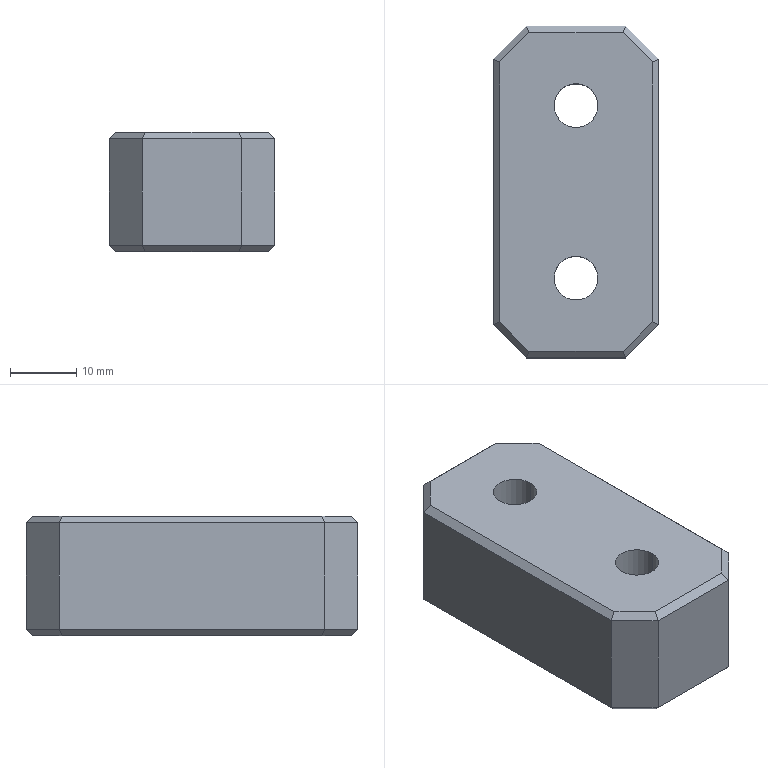Part | Creo | 1 solid | 36 faces | box 25 x 50 x 18 mm | volume 19381 mm3 | plane 28 | cylinder 8 | commonest cylinder face diameters 6.6 x4 11 x4
STEP:
#1=CARTESIAN_POINT('',(55.086,-82.005,-348.));
#2=VERTEX_POINT('',#1);
#3=CARTESIAN_POINT('',(40.914,-82.005,-348.));
#4=VERTEX_POINT('',#3);
#5=CARTESIAN_POINT('',(55.086,-82.005,-348.));
#6=DIRECTION('',(-1.,0.,0.));
#7=VECTOR('',#6,14.172);
#8=LINE('',#5,#7);
#9=EDGE_CURVE('',#2,#4,#8,.T.);
#10=ORIENTED_EDGE('',*,*,#9,.T.);
#11=CARTESIAN_POINT('',(36.5,-77.59,-348.));
#12=VERTEX_POINT('',#11);
#13=CARTESIAN_POINT('',(36.5,-77.59,-348.));
#14=DIRECTION('',(0.7071,-0.7071,0.));
#15=VECTOR('',#14,6.243);
#16=LINE('',#13,#15);
#17=EDGE_CURVE('',#12,#4,#16,.T.);
#18=ORIENTED_EDGE('',*,*,#17,.F.);
#19=CARTESIAN_POINT('',(36.5,-38.419,-348.));
#20=VERTEX_POINT('',#19);
#21=CARTESIAN_POINT('',(36.5,-77.59,-348.));
#22=DIRECTION('',(0.,1.,0.));
#23=VECTOR('',#22,39.172);
#24=LINE('',#21,#23);
#25=EDGE_CURVE('',#12,#20,#24,.T.);
#26=ORIENTED_EDGE('',*,*,#25,.T.);
#27=CARTESIAN_POINT('',(40.914,-34.005,-348.));
#28=VERTEX_POINT('',#27);
#29=CARTESIAN_POINT('',(40.914,-34.005,-348.));
#30=DIRECTION('',(-0.7071,-0.7071,0.));
#31=VECTOR('',#30,6.243);
#32=LINE('',#29,#31);
#33=EDGE_CURVE('',#28,#20,#32,.T.);
#34=ORIENTED_EDGE('',*,*,#33,.F.);
#35=CARTESIAN_POINT('',(55.086,-34.005,-348.));
#36=VERTEX_POINT('',#35);
#37=CARTESIAN_POINT('',(40.914,-34.005,-348.));
#38=DIRECTION('',(1.,0.,0.));
#39=VECTOR('',#38,14.172);
#40=LINE('',#37,#39);
#41=EDGE_CURVE('',#28,#36,#40,.T.);
#42=ORIENTED_EDGE('',*,*,#41,.T.);
#43=CARTESIAN_POINT('',(59.5,-38.419,-348.));
#44=VERTEX_POINT('',#43);
#45=CARTESIAN_POINT('',(59.5,-38.419,-348.));
#46=DIRECTION('',(-0.7071,0.7071,0.));
#47=VECTOR('',#46,6.243);
#48=LINE('',#45,#47);
#49=EDGE_CURVE('',#44,#36,#48,.T.);
#50=ORIENTED_EDGE('',*,*,#49,.F.);
#51=CARTESIAN_POINT('',(59.5,-77.59,-348.));
#52=VERTEX_POINT('',#51);
#53=CARTESIAN_POINT('',(59.5,-38.419,-348.));
#54=DIRECTION('',(0.,-1.,0.));
#55=VECTOR('',#54,39.172);
#56=LINE('',#53,#55);
#57=EDGE_CURVE('',#44,#52,#56,.T.);
#58=ORIENTED_EDGE('',*,*,#57,.T.);
#59=CARTESIAN_POINT('',(55.086,-82.005,-348.));
#60=DIRECTION('',(0.7071,0.7071,0.));
#61=VECTOR('',#60,6.243);
#62=LINE('',#59,#61);
#63=EDGE_CURVE('',#2,#52,#62,.T.);
#64=ORIENTED_EDGE('',*,*,#63,.F.);
#65=EDGE_LOOP('',(#10,#18,#26,#34,#42,#50,#58,#64));
#66=FACE_OUTER_BOUND('',#65,.F.);
#67=CARTESIAN_POINT('',(44.7,-71.005,-348.));
#68=VERTEX_POINT('',#67);
#69=CARTESIAN_POINT('',(51.3,-71.005,-348.));
#70=VERTEX_POINT('',#69);
#71=CARTESIAN_POINT('',(48.,-71.005,-348.));
#72=DIRECTION('',(0.,0.,-1.));
#73=DIRECTION('',(-1.,0.,0.));
#74=AXIS2_PLACEMENT_3D('',#71,#72,#73);
#75=CIRCLE('',#74,3.3);
#76=EDGE_CURVE('',#68,#70,#75,.T.);
#77=ORIENTED_EDGE('',*,*,#76,.F.);
#78=CARTESIAN_POINT('',(48.,-71.005,-348.));
#79=DIRECTION('',(0.,0.,-1.));
#80=DIRECTION('',(1.,0.,0.));
#81=AXIS2_PLACEMENT_3D('',#78,#79,#80);
#82=CIRCLE('',#81,3.3);
#83=EDGE_CURVE('',#70,#68,#82,.T.);
#84=ORIENTED_EDGE('',*,*,#83,.F.);
#85=EDGE_LOOP('',(#77,#84));
#86=FACE_BOUND('',#85,.F.);
#87=CARTESIAN_POINT('',(44.7,-45.005,-348.));
#88=VERTEX_POINT('',#87);
#89=CARTESIAN_POINT('',(51.3,-45.005,-348.));
#90=VERTEX_POINT('',#89);
#91=CARTESIAN_POINT('',(48.,-45.005,-348.));
#92=DIRECTION('',(0.,0.,-1.));
#93=DIRECTION('',(-1.,0.,0.));
#94=AXIS2_PLACEMENT_3D('',#91,#92,#93);
#95=CIRCLE('',#94,3.3);
#96=EDGE_CURVE('',#88,#90,#95,.T.);
#97=ORIENTED_EDGE('',*,*,#96,.F.);
#98=CARTESIAN_POINT('',(48.,-45.005,-348.));
#99=DIRECTION('',(0.,0.,-1.));
#100=DIRECTION('',(1.,0.,0.));
#101=AXIS2_PLACEMENT_3D('',#98,#99,#100);
#102=CIRCLE('',#101,3.3);
#103=EDGE_CURVE('',#90,#88,#102,.T.);
#104=ORIENTED_EDGE('',*,*,#103,.F.);
#105=EDGE_LOOP('',(#97,#104));
#106=FACE_BOUND('',#105,.F.);
#107=CARTESIAN_POINT('',(48.,-58.005,-348.));
#108=DIRECTION('',(0.,0.,1.));
#109=DIRECTION('',(0.,1.,0.));
#110=AXIS2_PLACEMENT_3D('',#107,#108,#109);
#111=PLANE('',#110);
#112=ADVANCED_FACE('',(#66,#86,#106),#111,.T.);
#113=ORIENTED_EDGE('',*,*,#76,.T.);
#114=CARTESIAN_POINT('',(51.3,-71.005,-359.));
#115=VERTEX_POINT('',#114);
#116=CARTESIAN_POINT('',(51.3,-71.005,-348.));
#117=DIRECTION('',(0.,0.,-1.));
#118=VECTOR('',#117,11.);
#119=LINE('',#116,#118);
#120=EDGE_CURVE('',#70,#115,#119,.T.);
#121=ORIENTED_EDGE('',*,*,#120,.T.);
#122=CARTESIAN_POINT('',(44.7,-71.005,-359.));
#123=VERTEX_POINT('',#122);
#124=CARTESIAN_POINT('',(48.,-71.005,-359.));
#125=DIRECTION('',(0.,0.,1.));
#126=DIRECTION('',(1.,0.,0.));
#127=AXIS2_PLACEMENT_3D('',#124,#125,#126);
#128=CIRCLE('',#127,3.3);
#129=EDGE_CURVE('',#115,#123,#128,.T.);
#130=ORIENTED_EDGE('',*,*,#129,.T.);
#131=CARTESIAN_POINT('',(44.7,-71.005,-348.));
#132=DIRECTION('',(0.,0.,-1.));
#133=VECTOR('',#132,11.);
#134=LINE('',#131,#133);
#135=EDGE_CURVE('',#68,#123,#134,.T.);
#136=ORIENTED_EDGE('',*,*,#135,.F.);
#137=EDGE_LOOP('',(#113,#121,#130,#136));
#138=FACE_OUTER_BOUND('',#137,.F.);
#139=CARTESIAN_POINT('',(48.,-71.005,-366.));
#140=DIRECTION('',(0.,0.,-1.));
#141=DIRECTION('',(-1.,0.,0.));
#142=AXIS2_PLACEMENT_3D('',#139,#140,#141);
#143=CYLINDRICAL_SURFACE('',#142,3.3);
#144=ADVANCED_FACE('',(#138),#143,.F.);
#145=ORIENTED_EDGE('',*,*,#83,.T.);
#146=ORIENTED_EDGE('',*,*,#135,.T.);
#147=CARTESIAN_POINT('',(48.,-71.005,-359.));
#148=DIRECTION('',(0.,0.,1.));
#149=DIRECTION('',(-1.,0.,0.));
#150=AXIS2_PLACEMENT_3D('',#147,#148,#149);
#151=CIRCLE('',#150,3.3);
#152=EDGE_CURVE('',#123,#115,#151,.T.);
#153=ORIENTED_EDGE('',*,*,#152,.T.);
#154=ORIENTED_EDGE('',*,*,#120,.F.);
#155=EDGE_LOOP('',(#145,#146,#153,#154));
#156=FACE_OUTER_BOUND('',#155,.F.);
#157=CARTESIAN_POINT('',(48.,-71.005,-366.));
#158=DIRECTION('',(0.,0.,-1.));
#159=DIRECTION('',(-1.,0.,0.));
#160=AXIS2_PLACEMENT_3D('',#157,#158,#159);
#161=CYLINDRICAL_SURFACE('',#160,3.3);
#162=ADVANCED_FACE('',(#156),#161,.F.);
#163=CARTESIAN_POINT('',(48.,-65.505,-359.));
#164=VERTEX_POINT('',#163);
#165=CARTESIAN_POINT('',(48.,-76.505,-359.));
#166=VERTEX_POINT('',#165);
#167=CARTESIAN_POINT('',(48.,-71.005,-359.));
#168=DIRECTION('',(0.,0.,-1.));
#169=DIRECTION('',(0.,1.,0.));
#170=AXIS2_PLACEMENT_3D('',#167,#168,#169);
#171=CIRCLE('',#170,5.5);
#172=EDGE_CURVE('',#164,#166,#171,.T.);
#173=ORIENTED_EDGE('',*,*,#172,.F.);
#174=CARTESIAN_POINT('',(48.,-71.005,-359.));
#175=DIRECTION('',(0.,0.,-1.));
#176=DIRECTION('',(0.,-1.,0.));
#177=AXIS2_PLACEMENT_3D('',#174,#175,#176);
#178=CIRCLE('',#177,5.5);
#179=EDGE_CURVE('',#166,#164,#178,.T.);
#180=ORIENTED_EDGE('',*,*,#179,.F.);
#181=EDGE_LOOP('',(#173,#180));
#182=FACE_OUTER_BOUND('',#181,.F.);
#183=ORIENTED_EDGE('',*,*,#152,.F.);
#184=ORIENTED_EDGE('',*,*,#129,.F.);
#185=EDGE_LOOP('',(#183,#184));
#186=FACE_BOUND('',#185,.F.);
#187=CARTESIAN_POINT('',(48.,-71.005,-359.));
#188=DIRECTION('',(0.,0.,1.));
#189=DIRECTION('',(0.,1.,0.));
#190=AXIS2_PLACEMENT_3D('',#187,#188,#189);
#191=PLANE('',#190);
#192=ADVANCED_FACE('',(#182,#186),#191,.F.);
#193=ORIENTED_EDGE('',*,*,#172,.T.);
#194=CARTESIAN_POINT('',(48.,-76.505,-366.));
#195=VERTEX_POINT('',#194);
#196=CARTESIAN_POINT('',(48.,-76.505,-366.));
#197=DIRECTION('',(0.,0.,1.));
#198=VECTOR('',#197,7.);
#199=LINE('',#196,#198);
#200=EDGE_CURVE('',#195,#166,#199,.T.);
#201=ORIENTED_EDGE('',*,*,#200,.F.);
#202=CARTESIAN_POINT('',(53.5,-71.005,-366.));
#203=VERTEX_POINT('',#202);
#204=CARTESIAN_POINT('',(48.,-71.005,-366.));
#205=DIRECTION('',(0.,0.,1.));
#206=DIRECTION('',(0.,-1.,0.));
#207=AXIS2_PLACEMENT_3D('',#204,#205,#206);
#208=CIRCLE('',#207,5.5);
#209=EDGE_CURVE('',#195,#203,#208,.T.);
#210=ORIENTED_EDGE('',*,*,#209,.T.);
#211=CARTESIAN_POINT('',(48.,-65.505,-366.));
#212=VERTEX_POINT('',#211);
#213=CARTESIAN_POINT('',(48.,-71.005,-366.));
#214=DIRECTION('',(0.,0.,1.));
#215=DIRECTION('',(1.,0.,0.));
#216=AXIS2_PLACEMENT_3D('',#213,#214,#215);
#217=CIRCLE('',#216,5.5);
#218=EDGE_CURVE('',#203,#212,#217,.T.);
#219=ORIENTED_EDGE('',*,*,#218,.T.);
#220=CARTESIAN_POINT('',(48.,-65.505,-366.));
#221=DIRECTION('',(0.,0.,1.));
#222=VECTOR('',#221,7.);
#223=LINE('',#220,#222);
#224=EDGE_CURVE('',#212,#164,#223,.T.);
#225=ORIENTED_EDGE('',*,*,#224,.T.);
#226=EDGE_LOOP('',(#193,#201,#210,#219,#225));
#227=FACE_OUTER_BOUND('',#226,.F.);
#228=CARTESIAN_POINT('',(48.,-71.005,-372.));
#229=DIRECTION('',(0.,0.,1.));
#230=DIRECTION('',(0.,1.,0.));
#231=AXIS2_PLACEMENT_3D('',#228,#229,#230);
#232=CYLINDRICAL_SURFACE('',#231,5.5);
#233=ADVANCED_FACE('',(#227),#232,.F.);
#234=ORIENTED_EDGE('',*,*,#179,.T.);
#235=ORIENTED_EDGE('',*,*,#224,.F.);
#236=CARTESIAN_POINT('',(42.5,-71.005,-366.));
#237=VERTEX_POINT('',#236);
#238=CARTESIAN_POINT('',(48.,-71.005,-366.));
#239=DIRECTION('',(0.,0.,1.));
#240=DIRECTION('',(0.,1.,0.));
#241=AXIS2_PLACEMENT_3D('',#238,#239,#240);
#242=CIRCLE('',#241,5.5);
#243=EDGE_CURVE('',#212,#237,#242,.T.);
#244=ORIENTED_EDGE('',*,*,#243,.T.);
#245=CARTESIAN_POINT('',(48.,-71.005,-366.));
#246=DIRECTION('',(0.,0.,1.));
#247=DIRECTION('',(-1.,0.,0.));
#248=AXIS2_PLACEMENT_3D('',#245,#246,#247);
#249=CIRCLE('',#248,5.5);
#250=EDGE_CURVE('',#237,#195,#249,.T.);
#251=ORIENTED_EDGE('',*,*,#250,.T.);
#252=ORIENTED_EDGE('',*,*,#200,.T.);
#253=EDGE_LOOP('',(#234,#235,#244,#251,#252));
#254=FACE_OUTER_BOUND('',#253,.F.);
#255=CARTESIAN_POINT('',(48.,-71.005,-372.));
#256=DIRECTION('',(0.,0.,1.));
#257=DIRECTION('',(0.,1.,0.));
#258=AXIS2_PLACEMENT_3D('',#255,#256,#257);
#259=CYLINDRICAL_SURFACE('',#258,5.5);
#260=ADVANCED_FACE('',(#254),#259,.F.);
#261=CARTESIAN_POINT('',(59.5,-77.59,-366.));
#262=VERTEX_POINT('',#261);
#263=CARTESIAN_POINT('',(59.5,-38.419,-366.));
#264=VERTEX_POINT('',#263);
#265=CARTESIAN_POINT('',(59.5,-77.59,-366.));
#266=DIRECTION('',(0.,1.,0.));
#267=VECTOR('',#266,39.172);
#268=LINE('',#265,#267);
#269=EDGE_CURVE('',#262,#264,#268,.T.);
#270=ORIENTED_EDGE('',*,*,#269,.T.);
#271=CARTESIAN_POINT('',(55.086,-34.005,-366.));
#272=VERTEX_POINT('',#271);
#273=CARTESIAN_POINT('',(55.086,-34.005,-366.));
#274=DIRECTION('',(0.7071,-0.7071,0.));
#275=VECTOR('',#274,6.243);
#276=LINE('',#273,#275);
#277=EDGE_CURVE('',#272,#264,#276,.T.);
#278=ORIENTED_EDGE('',*,*,#277,.F.);
#279=CARTESIAN_POINT('',(40.914,-34.005,-366.));
#280=VERTEX_POINT('',#279);
#281=CARTESIAN_POINT('',(55.086,-34.005,-366.));
#282=DIRECTION('',(-1.,0.,0.));
#283=VECTOR('',#282,14.172);
#284=LINE('',#281,#283);
#285=EDGE_CURVE('',#272,#280,#284,.T.);
#286=ORIENTED_EDGE('',*,*,#285,.T.);
#287=CARTESIAN_POINT('',(36.5,-38.419,-366.));
#288=VERTEX_POINT('',#287);
#289=CARTESIAN_POINT('',(36.5,-38.419,-366.));
#290=DIRECTION('',(0.7071,0.7071,0.));
#291=VECTOR('',#290,6.243);
#292=LINE('',#289,#291);
#293=EDGE_CURVE('',#288,#280,#292,.T.);
#294=ORIENTED_EDGE('',*,*,#293,.F.);
#295=CARTESIAN_POINT('',(36.5,-77.59,-366.));
#296=VERTEX_POINT('',#295);
#297=CARTESIAN_POINT('',(36.5,-38.419,-366.));
#298=DIRECTION('',(0.,-1.,0.));
#299=VECTOR('',#298,39.172);
#300=LINE('',#297,#299);
#301=EDGE_CURVE('',#288,#296,#300,.T.);
#302=ORIENTED_EDGE('',*,*,#301,.T.);
#303=CARTESIAN_POINT('',(40.914,-82.005,-366.));
#304=VERTEX_POINT('',#303);
#305=CARTESIAN_POINT('',(40.914,-82.005,-366.));
#306=DIRECTION('',(-0.7071,0.7071,0.));
#307=VECTOR('',#306,6.243);
#308=LINE('',#305,#307);
#309=EDGE_CURVE('',#304,#296,#308,.T.);
#310=ORIENTED_EDGE('',*,*,#309,.F.);
#311=CARTESIAN_POINT('',(55.086,-82.005,-366.));
#312=VERTEX_POINT('',#311);
#313=CARTESIAN_POINT('',(40.914,-82.005,-366.));
#314=DIRECTION('',(1.,0.,0.));
#315=VECTOR('',#314,14.172);
#316=LINE('',#313,#315);
#317=EDGE_CURVE('',#304,#312,#316,.T.);
#318=ORIENTED_EDGE('',*,*,#317,.T.);
#319=CARTESIAN_POINT('',(59.5,-77.59,-366.));
#320=DIRECTION('',(-0.7071,-0.7071,0.));
#321=VECTOR('',#320,6.243);
#322=LINE('',#319,#321);
#323=EDGE_CURVE('',#262,#312,#322,.T.);
#324=ORIENTED_EDGE('',*,*,#323,.F.);
#325=EDGE_LOOP('',(#270,#278,#286,#294,#302,#310,#318,#324));
#326=FACE_OUTER_BOUND('',#325,.F.);
#327=CARTESIAN_POINT('',(53.5,-45.005,-366.));
#328=VERTEX_POINT('',#327);
#329=CARTESIAN_POINT('',(48.,-39.505,-366.));
#330=VERTEX_POINT('',#329);
#331=CARTESIAN_POINT('',(48.,-45.005,-366.));
#332=DIRECTION('',(0.,0.,1.));
#333=DIRECTION('',(1.,0.,0.));
#334=AXIS2_PLACEMENT_3D('',#331,#332,#333);
#335=CIRCLE('',#334,5.5);
#336=EDGE_CURVE('',#328,#330,#335,.T.);
#337=ORIENTED_EDGE('',*,*,#336,.F.);
#338=CARTESIAN_POINT('',(48.,-50.505,-366.));
#339=VERTEX_POINT('',#338);
#340=CARTESIAN_POINT('',(48.,-45.005,-366.));
#341=DIRECTION('',(0.,0.,1.));
#342=DIRECTION('',(0.,-1.,0.));
#343=AXIS2_PLACEMENT_3D('',#340,#341,#342);
#344=CIRCLE('',#343,5.5);
#345=EDGE_CURVE('',#339,#328,#344,.T.);
#346=ORIENTED_EDGE('',*,*,#345,.F.);
#347=CARTESIAN_POINT('',(42.5,-45.005,-366.));
#348=VERTEX_POINT('',#347);
#349=CARTESIAN_POINT('',(48.,-45.005,-366.));
#350=DIRECTION('',(0.,0.,1.));
#351=DIRECTION('',(-1.,0.,0.));
#352=AXIS2_PLACEMENT_3D('',#349,#350,#351);
#353=CIRCLE('',#352,5.5);
#354=EDGE_CURVE('',#348,#339,#353,.T.);
#355=ORIENTED_EDGE('',*,*,#354,.F.);
#356=CARTESIAN_POINT('',(48.,-45.005,-366.));
#357=DIRECTION('',(0.,0.,1.));
#358=DIRECTION('',(0.,1.,0.));
#359=AXIS2_PLACEMENT_3D('',#356,#357,#358);
#360=CIRCLE('',#359,5.5);
#361=EDGE_CURVE('',#330,#348,#360,.T.);
#362=ORIENTED_EDGE('',*,*,#361,.F.);
#363=EDGE_LOOP('',(#337,#346,#355,#362));
#364=FACE_BOUND('',#363,.F.);
#365=ORIENTED_EDGE('',*,*,#218,.F.);
#366=ORIENTED_EDGE('',*,*,#209,.F.);
#367=ORIENTED_EDGE('',*,*,#250,.F.);
#368=ORIENTED_EDGE('',*,*,#243,.F.);
#369=EDGE_LOOP('',(#365,#366,#367,#368));
#370=FACE_BOUND('',#369,.F.);
#371=CARTESIAN_POINT('',(10.,-0.004699,-366.));
#372=DIRECTION('',(0.,0.,1.));
#373=DIRECTION('',(0.,1.,0.));
#374=AXIS2_PLACEMENT_3D('',#371,#372,#373);
#375=PLANE('',#374);
#376=ADVANCED_FACE('',(#326,#364,#370),#375,.F.);
#377=CARTESIAN_POINT('',(60.5,-38.005,-365.));
#378=VERTEX_POINT('',#377);
#379=CARTESIAN_POINT('',(60.5,-38.005,-365.));
#380=DIRECTION('',(-0.6786,-0.2811,-0.6786));
#381=VECTOR('',#380,1.474);
#382=LINE('',#379,#381);
#383=EDGE_CURVE('',#378,#264,#382,.T.);
#384=ORIENTED_EDGE('',*,*,#383,.T.);
#385=ORIENTED_EDGE('',*,*,#269,.F.);
#386=CARTESIAN_POINT('',(60.5,-78.005,-365.));
#387=VERTEX_POINT('',#386);
#388=CARTESIAN_POINT('',(60.5,-78.005,-365.));
#389=DIRECTION('',(-0.6786,0.2811,-0.6786));
#390=VECTOR('',#389,1.474);
#391=LINE('',#388,#390);
#392=EDGE_CURVE('',#387,#262,#391,.T.);
#393=ORIENTED_EDGE('',*,*,#392,.F.);
#394=CARTESIAN_POINT('',(60.5,-38.005,-365.));
#395=DIRECTION('',(0.,-1.,0.));
#396=VECTOR('',#395,40.);
#397=LINE('',#394,#396);
#398=EDGE_CURVE('',#378,#387,#397,.T.);
#399=ORIENTED_EDGE('',*,*,#398,.F.);
#400=EDGE_LOOP('',(#384,#385,#393,#399));
#401=FACE_OUTER_BOUND('',#400,.F.);
#402=CARTESIAN_POINT('',(60.5,-88.005,-365.));
#403=DIRECTION('',(0.7071,0.,-0.7071));
#404=DIRECTION('',(0.,1.,0.));
#405=AXIS2_PLACEMENT_3D('',#402,#403,#404);
#406=PLANE('',#405);
#407=ADVANCED_FACE('',(#401),#406,.T.);
#408=CARTESIAN_POINT('',(55.5,-33.005,-365.));
#409=VERTEX_POINT('',#408);
#410=CARTESIAN_POINT('',(55.5,-33.005,-365.));
#411=DIRECTION('',(-0.2811,-0.6786,-0.6786));
#412=VECTOR('',#411,1.474);
#413=LINE('',#410,#412);
#414=EDGE_CURVE('',#409,#272,#413,.T.);
#415=ORIENTED_EDGE('',*,*,#414,.T.);
#416=ORIENTED_EDGE('',*,*,#277,.T.);
#417=ORIENTED_EDGE('',*,*,#383,.F.);
#418=CARTESIAN_POINT('',(55.5,-33.005,-365.));
#419=DIRECTION('',(0.7071,-0.7071,0.));
#420=VECTOR('',#419,7.071);
#421=LINE('',#418,#420);
#422=EDGE_CURVE('',#409,#378,#421,.T.);
#423=ORIENTED_EDGE('',*,*,#422,.F.);
#424=EDGE_LOOP('',(#415,#416,#417,#423));
#425=FACE_OUTER_BOUND('',#424,.F.);
#426=CARTESIAN_POINT('',(15.543,5.538,-366.));
#427=DIRECTION('',(-0.5,-0.5,0.7071));
#428=DIRECTION('',(-0.7071,0.7071,0.));
#429=AXIS2_PLACEMENT_3D('',#426,#427,#428);
#430=PLANE('',#429);
#431=ADVANCED_FACE('',(#425),#430,.F.);
#432=CARTESIAN_POINT('',(40.5,-33.005,-365.));
#433=VERTEX_POINT('',#432);
#434=CARTESIAN_POINT('',(40.5,-33.005,-365.));
#435=DIRECTION('',(0.2811,-0.6786,-0.6786));
#436=VECTOR('',#435,1.474);
#437=LINE('',#434,#436);
#438=EDGE_CURVE('',#433,#280,#437,.T.);
#439=ORIENTED_EDGE('',*,*,#438,.T.);
#440=ORIENTED_EDGE('',*,*,#285,.F.);
#441=ORIENTED_EDGE('',*,*,#414,.F.);
#442=CARTESIAN_POINT('',(40.5,-33.005,-365.));
#443=DIRECTION('',(1.,0.,0.));
#444=VECTOR('',#443,15.);
#445=LINE('',#442,#444);
#446=EDGE_CURVE('',#433,#409,#445,.T.);
#447=ORIENTED_EDGE('',*,*,#446,.F.);
#448=EDGE_LOOP('',(#439,#440,#441,#447));
#449=FACE_OUTER_BOUND('',#448,.F.);
#450=CARTESIAN_POINT('',(63.,-33.005,-365.));
#451=DIRECTION('',(0.,0.7071,-0.7071));
#452=DIRECTION('',(-1.,0.,0.));
#453=AXIS2_PLACEMENT_3D('',#450,#451,#452);
#454=PLANE('',#453);
#455=ADVANCED_FACE('',(#449),#454,.T.);
#456=CARTESIAN_POINT('',(35.5,-38.005,-365.));
#457=VERTEX_POINT('',#456);
#458=CARTESIAN_POINT('',(36.5,-38.419,-366.));
#459=DIRECTION('',(-0.6786,0.2811,0.6786));
#460=VECTOR('',#459,1.474);
#461=LINE('',#458,#460);
#462=EDGE_CURVE('',#288,#457,#461,.T.);
#463=ORIENTED_EDGE('',*,*,#462,.F.);
#464=ORIENTED_EDGE('',*,*,#293,.T.);
#465=ORIENTED_EDGE('',*,*,#438,.F.);
#466=CARTESIAN_POINT('',(35.5,-38.005,-365.));
#467=DIRECTION('',(0.7071,0.7071,0.));
#468=VECTOR('',#467,7.071);
#469=LINE('',#466,#468);
#470=EDGE_CURVE('',#457,#433,#469,.T.);
#471=ORIENTED_EDGE('',*,*,#470,.F.);
#472=EDGE_LOOP('',(#463,#464,#465,#471));
#473=FACE_OUTER_BOUND('',#472,.F.);
#474=CARTESIAN_POINT('',(42.457,-32.462,-366.));
#475=DIRECTION('',(0.5,-0.5,0.7071));
#476=DIRECTION('',(-0.7071,-0.7071,0.));
#477=AXIS2_PLACEMENT_3D('',#474,#475,#476);
#478=PLANE('',#477);
#479=ADVANCED_FACE('',(#473),#478,.F.);
#480=ORIENTED_EDGE('',*,*,#462,.T.);
#481=CARTESIAN_POINT('',(35.5,-78.005,-365.));
#482=VERTEX_POINT('',#481);
#483=CARTESIAN_POINT('',(35.5,-78.005,-365.));
#484=DIRECTION('',(0.,1.,0.));
#485=VECTOR('',#484,40.);
#486=LINE('',#483,#485);
#487=EDGE_CURVE('',#482,#457,#486,.T.);
#488=ORIENTED_EDGE('',*,*,#487,.F.);
#489=CARTESIAN_POINT('',(36.5,-77.59,-366.));
#490=DIRECTION('',(-0.6786,-0.2811,0.6786));
#491=VECTOR('',#490,1.474);
#492=LINE('',#489,#491);
#493=EDGE_CURVE('',#296,#482,#492,.T.);
#494=ORIENTED_EDGE('',*,*,#493,.F.);
#495=ORIENTED_EDGE('',*,*,#301,.F.);
#496=EDGE_LOOP('',(#480,#488,#494,#495));
#497=FACE_OUTER_BOUND('',#496,.F.);
#498=CARTESIAN_POINT('',(35.5,-28.005,-365.));
#499=DIRECTION('',(-0.7071,0.,-0.7071));
#500=DIRECTION('',(0.,-1.,0.));
#501=AXIS2_PLACEMENT_3D('',#498,#499,#500);
#502=PLANE('',#501);
#503=ADVANCED_FACE('',(#497),#502,.T.);
#504=CARTESIAN_POINT('',(35.5,-38.005,-349.));
#505=VERTEX_POINT('',#504);
#506=CARTESIAN_POINT('',(35.5,-38.005,-365.));
#507=DIRECTION('',(0.,0.,1.));
#508=VECTOR('',#507,16.);
#509=LINE('',#506,#508);
#510=EDGE_CURVE('',#457,#505,#509,.T.);
#511=ORIENTED_EDGE('',*,*,#510,.T.);
#512=CARTESIAN_POINT('',(35.5,-78.005,-349.));
#513=VERTEX_POINT('',#512);
#514=CARTESIAN_POINT('',(35.5,-38.005,-349.));
#515=DIRECTION('',(0.,-1.,0.));
#516=VECTOR('',#515,40.);
#517=LINE('',#514,#516);
#518=EDGE_CURVE('',#505,#513,#517,.T.);
#519=ORIENTED_EDGE('',*,*,#518,.T.);
#520=CARTESIAN_POINT('',(35.5,-78.005,-349.));
#521=DIRECTION('',(0.,0.,-1.));
#522=VECTOR('',#521,16.);
#523=LINE('',#520,#522);
#524=EDGE_CURVE('',#513,#482,#523,.T.);
#525=ORIENTED_EDGE('',*,*,#524,.T.);
#526=ORIENTED_EDGE('',*,*,#487,.T.);
#527=EDGE_LOOP('',(#511,#519,#525,#526));
#528=FACE_OUTER_BOUND('',#527,.F.);
#529=CARTESIAN_POINT('',(35.5,-28.005,-354.));
#530=DIRECTION('',(-1.,0.,0.));
#531=DIRECTION('',(0.,-1.,0.));
#532=AXIS2_PLACEMENT_3D('',#529,#530,#531);
#533=PLANE('',#532);
#534=ADVANCED_FACE('',(#528),#533,.T.);
#535=CARTESIAN_POINT('',(40.5,-33.005,-349.));
#536=VERTEX_POINT('',#535);
#537=CARTESIAN_POINT('',(40.5,-33.005,-349.));
#538=DIRECTION('',(0.,0.,-1.));
#539=VECTOR('',#538,16.);
#540=LINE('',#537,#539);
#541=EDGE_CURVE('',#536,#433,#540,.T.);
#542=ORIENTED_EDGE('',*,*,#541,.F.);
#543=CARTESIAN_POINT('',(40.5,-33.005,-349.));
#544=DIRECTION('',(-0.7071,-0.7071,0.));
#545=VECTOR('',#544,7.071);
#546=LINE('',#543,#545);
#547=EDGE_CURVE('',#536,#505,#546,.T.);
#548=ORIENTED_EDGE('',*,*,#547,.T.);
#549=ORIENTED_EDGE('',*,*,#510,.F.);
#550=ORIENTED_EDGE('',*,*,#470,.T.);
#551=EDGE_LOOP('',(#542,#548,#549,#550));
#552=FACE_OUTER_BOUND('',#551,.F.);
#553=CARTESIAN_POINT('',(40.5,-33.005,-354.));
#554=DIRECTION('',(0.7071,-0.7071,0.));
#555=DIRECTION('',(0.,0.,-1.));
#556=AXIS2_PLACEMENT_3D('',#553,#554,#555);
#557=PLANE('',#556);
#558=ADVANCED_FACE('',(#552),#557,.F.);
#559=CARTESIAN_POINT('',(55.5,-33.005,-349.));
#560=VERTEX_POINT('',#559);
#561=CARTESIAN_POINT('',(55.5,-33.005,-365.));
#562=DIRECTION('',(0.,0.,1.));
#563=VECTOR('',#562,16.);
#564=LINE('',#561,#563);
#565=EDGE_CURVE('',#409,#560,#564,.T.);
#566=ORIENTED_EDGE('',*,*,#565,.T.);
#567=CARTESIAN_POINT('',(55.5,-33.005,-349.));
#568=DIRECTION('',(-1.,0.,0.));
#569=VECTOR('',#568,15.);
#570=LINE('',#567,#569);
#571=EDGE_CURVE('',#560,#536,#570,.T.);
#572=ORIENTED_EDGE('',*,*,#571,.T.);
#573=ORIENTED_EDGE('',*,*,#541,.T.);
#574=ORIENTED_EDGE('',*,*,#446,.T.);
#575=EDGE_LOOP('',(#566,#572,#573,#574));
#576=FACE_OUTER_BOUND('',#575,.F.);
#577=CARTESIAN_POINT('',(63.,-33.005,-354.));
#578=DIRECTION('',(0.,1.,0.));
#579=DIRECTION('',(-1.,0.,0.));
#580=AXIS2_PLACEMENT_3D('',#577,#578,#579);
#581=PLANE('',#580);
#582=ADVANCED_FACE('',(#576),#581,.T.);
#583=CARTESIAN_POINT('',(60.5,-38.005,-349.));
#584=VERTEX_POINT('',#583);
#585=CARTESIAN_POINT('',(60.5,-38.005,-349.));
#586=DIRECTION('',(0.,0.,-1.));
#587=VECTOR('',#586,16.);
#588=LINE('',#585,#587);
#589=EDGE_CURVE('',#584,#378,#588,.T.);
#590=ORIENTED_EDGE('',*,*,#589,.F.);
#591=CARTESIAN_POINT('',(60.5,-38.005,-349.));
#592=DIRECTION('',(-0.7071,0.7071,0.));
#593=VECTOR('',#592,7.071);
#594=LINE('',#591,#593);
#595=EDGE_CURVE('',#584,#560,#594,.T.);
#596=ORIENTED_EDGE('',*,*,#595,.T.);
#597=ORIENTED_EDGE('',*,*,#565,.F.);
#598=ORIENTED_EDGE('',*,*,#422,.T.);
#599=EDGE_LOOP('',(#590,#596,#597,#598));
#600=FACE_OUTER_BOUND('',#599,.F.);
#601=CARTESIAN_POINT('',(60.5,-38.005,-354.));
#602=DIRECTION('',(-0.7071,-0.7071,0.));
#603=DIRECTION('',(0.,0.,-1.));
#604=AXIS2_PLACEMENT_3D('',#601,#602,#603);
#605=PLANE('',#604);
#606=ADVANCED_FACE('',(#600),#605,.F.);
#607=CARTESIAN_POINT('',(60.5,-78.005,-349.));
#608=VERTEX_POINT('',#607);
#609=CARTESIAN_POINT('',(60.5,-78.005,-365.));
#610=DIRECTION('',(0.,0.,1.));
#611=VECTOR('',#610,16.);
#612=LINE('',#609,#611);
#613=EDGE_CURVE('',#387,#608,#612,.T.);
#614=ORIENTED_EDGE('',*,*,#613,.T.);
#615=CARTESIAN_POINT('',(60.5,-78.005,-349.));
#616=DIRECTION('',(0.,1.,0.));
#617=VECTOR('',#616,40.);
#618=LINE('',#615,#617);
#619=EDGE_CURVE('',#608,#584,#618,.T.);
#620=ORIENTED_EDGE('',*,*,#619,.T.);
#621=ORIENTED_EDGE('',*,*,#589,.T.);
#622=ORIENTED_EDGE('',*,*,#398,.T.);
#623=EDGE_LOOP('',(#614,#620,#621,#622));
#624=FACE_OUTER_BOUND('',#623,.F.);
#625=CARTESIAN_POINT('',(60.5,-88.005,-354.));
#626=DIRECTION('',(1.,0.,0.));
#627=DIRECTION('',(0.,1.,0.));
#628=AXIS2_PLACEMENT_3D('',#625,#626,#627);
#629=PLANE('',#628);
#630=ADVANCED_FACE('',(#624),#629,.T.);
#631=CARTESIAN_POINT('',(55.5,-83.005,-349.));
#632=VERTEX_POINT('',#631);
#633=CARTESIAN_POINT('',(55.5,-83.005,-365.));
#634=VERTEX_POINT('',#633);
#635=CARTESIAN_POINT('',(55.5,-83.005,-349.));
#636=DIRECTION('',(0.,0.,-1.));
#637=VECTOR('',#636,16.);
#638=LINE('',#635,#637);
#639=EDGE_CURVE('',#632,#634,#638,.T.);
#640=ORIENTED_EDGE('',*,*,#639,.F.);
#641=CARTESIAN_POINT('',(55.5,-83.005,-349.));
#642=DIRECTION('',(0.7071,0.7071,0.));
#643=VECTOR('',#642,7.071);
#644=LINE('',#641,#643);
#645=EDGE_CURVE('',#632,#608,#644,.T.);
#646=ORIENTED_EDGE('',*,*,#645,.T.);
#647=ORIENTED_EDGE('',*,*,#613,.F.);
#648=CARTESIAN_POINT('',(60.5,-78.005,-365.));
#649=DIRECTION('',(-0.7071,-0.7071,0.));
#650=VECTOR('',#649,7.071);
#651=LINE('',#648,#650);
#652=EDGE_CURVE('',#387,#634,#651,.T.);
#653=ORIENTED_EDGE('',*,*,#652,.T.);
#654=EDGE_LOOP('',(#640,#646,#647,#653));
#655=FACE_OUTER_BOUND('',#654,.F.);
#656=CARTESIAN_POINT('',(55.5,-83.005,-354.));
#657=DIRECTION('',(-0.7071,0.7071,0.));
#658=DIRECTION('',(0.,0.,-1.));
#659=AXIS2_PLACEMENT_3D('',#656,#657,#658);
#660=PLANE('',#659);
#661=ADVANCED_FACE('',(#655),#660,.F.);
#662=CARTESIAN_POINT('',(40.5,-83.005,-365.));
#663=VERTEX_POINT('',#662);
#664=CARTESIAN_POINT('',(40.5,-83.005,-349.));
#665=VERTEX_POINT('',#664);
#666=CARTESIAN_POINT('',(40.5,-83.005,-365.));
#667=DIRECTION('',(0.,0.,1.));
#668=VECTOR('',#667,16.);
#669=LINE('',#666,#668);
#670=EDGE_CURVE('',#663,#665,#669,.T.);
#671=ORIENTED_EDGE('',*,*,#670,.T.);
#672=CARTESIAN_POINT('',(40.5,-83.005,-349.));
#673=DIRECTION('',(1.,0.,0.));
#674=VECTOR('',#673,15.);
#675=LINE('',#672,#674);
#676=EDGE_CURVE('',#665,#632,#675,.T.);
#677=ORIENTED_EDGE('',*,*,#676,.T.);
#678=ORIENTED_EDGE('',*,*,#639,.T.);
#679=CARTESIAN_POINT('',(55.5,-83.005,-365.));
#680=DIRECTION('',(-1.,0.,0.));
#681=VECTOR('',#680,15.);
#682=LINE('',#679,#681);
#683=EDGE_CURVE('',#634,#663,#682,.T.);
#684=ORIENTED_EDGE('',*,*,#683,.T.);
#685=EDGE_LOOP('',(#671,#677,#678,#684));
#686=FACE_OUTER_BOUND('',#685,.F.);
#687=CARTESIAN_POINT('',(33.,-83.005,-354.));
#688=DIRECTION('',(0.,-1.,0.));
#689=DIRECTION('',(1.,0.,0.));
#690=AXIS2_PLACEMENT_3D('',#687,#688,#689);
#691=PLANE('',#690);
#692=ADVANCED_FACE('',(#686),#691,.T.);
#693=ORIENTED_EDGE('',*,*,#524,.F.);
#694=CARTESIAN_POINT('',(35.5,-78.005,-349.));
#695=DIRECTION('',(0.7071,-0.7071,0.));
#696=VECTOR('',#695,7.071);
#697=LINE('',#694,#696);
#698=EDGE_CURVE('',#513,#665,#697,.T.);
#699=ORIENTED_EDGE('',*,*,#698,.T.);
#700=ORIENTED_EDGE('',*,*,#670,.F.);
#701=CARTESIAN_POINT('',(40.5,-83.005,-365.));
#702=DIRECTION('',(-0.7071,0.7071,0.));
#703=VECTOR('',#702,7.071);
#704=LINE('',#701,#703);
#705=EDGE_CURVE('',#663,#482,#704,.T.);
#706=ORIENTED_EDGE('',*,*,#705,.T.);
#707=EDGE_LOOP('',(#693,#699,#700,#706));
#708=FACE_OUTER_BOUND('',#707,.F.);
#709=CARTESIAN_POINT('',(35.5,-78.005,-354.));
#710=DIRECTION('',(0.7071,0.7071,0.));
#711=DIRECTION('',(0.,0.,-1.));
#712=AXIS2_PLACEMENT_3D('',#709,#710,#711);
#713=PLANE('',#712);
#714=ADVANCED_FACE('',(#708),#713,.F.);
#715=CARTESIAN_POINT('',(35.5,-78.005,-349.));
#716=DIRECTION('',(0.6786,0.2811,0.6786));
#717=VECTOR('',#716,1.474);
#718=LINE('',#715,#717);
#719=EDGE_CURVE('',#513,#12,#718,.T.);
#720=ORIENTED_EDGE('',*,*,#719,.T.);
#721=ORIENTED_EDGE('',*,*,#17,.T.);
#722=CARTESIAN_POINT('',(40.5,-83.005,-349.));
#723=DIRECTION('',(0.2811,0.6786,0.6786));
#724=VECTOR('',#723,1.474);
#725=LINE('',#722,#724);
#726=EDGE_CURVE('',#665,#4,#725,.T.);
#727=ORIENTED_EDGE('',*,*,#726,.F.);
#728=ORIENTED_EDGE('',*,*,#698,.F.);
#729=EDGE_LOOP('',(#720,#721,#727,#728));
#730=FACE_OUTER_BOUND('',#729,.F.);
#731=CARTESIAN_POINT('',(32.457,-73.548,-348.));
#732=DIRECTION('',(-0.5,-0.5,0.7071));
#733=DIRECTION('',(0.7071,-0.7071,0.));
#734=AXIS2_PLACEMENT_3D('',#731,#732,#733);
#735=PLANE('',#734);
#736=ADVANCED_FACE('',(#730),#735,.T.);
#737=CARTESIAN_POINT('',(35.5,-38.005,-349.));
#738=DIRECTION('',(0.6786,-0.2811,0.6786));
#739=VECTOR('',#738,1.474);
#740=LINE('',#737,#739);
#741=EDGE_CURVE('',#505,#20,#740,.T.);
#742=ORIENTED_EDGE('',*,*,#741,.T.);
#743=ORIENTED_EDGE('',*,*,#25,.F.);
#744=ORIENTED_EDGE('',*,*,#719,.F.);
#745=ORIENTED_EDGE('',*,*,#518,.F.);
#746=EDGE_LOOP('',(#742,#743,#744,#745));
#747=FACE_OUTER_BOUND('',#746,.F.);
#748=CARTESIAN_POINT('',(35.5,-28.005,-349.));
#749=DIRECTION('',(0.7071,0.,-0.7071));
#750=DIRECTION('',(0.,-1.,0.));
#751=AXIS2_PLACEMENT_3D('',#748,#749,#750);
#752=PLANE('',#751);
#753=ADVANCED_FACE('',(#747),#752,.F.);
#754=CARTESIAN_POINT('',(40.5,-33.005,-349.));
#755=DIRECTION('',(0.2811,-0.6786,0.6786));
#756=VECTOR('',#755,1.474);
#757=LINE('',#754,#756);
#758=EDGE_CURVE('',#536,#28,#757,.T.);
#759=ORIENTED_EDGE('',*,*,#758,.T.);
#760=ORIENTED_EDGE('',*,*,#33,.T.);
#761=ORIENTED_EDGE('',*,*,#741,.F.);
#762=ORIENTED_EDGE('',*,*,#547,.F.);
#763=EDGE_LOOP('',(#759,#760,#761,#762));
#764=FACE_OUTER_BOUND('',#763,.F.);
#765=CARTESIAN_POINT('',(32.457,-42.462,-348.));
#766=DIRECTION('',(-0.5,0.5,0.7071));
#767=DIRECTION('',(-0.7071,-0.7071,0.));
#768=AXIS2_PLACEMENT_3D('',#765,#766,#767);
#769=PLANE('',#768);
#770=ADVANCED_FACE('',(#764),#769,.T.);
#771=ORIENTED_EDGE('',*,*,#758,.F.);
#772=ORIENTED_EDGE('',*,*,#571,.F.);
#773=CARTESIAN_POINT('',(55.086,-34.005,-348.));
#774=DIRECTION('',(0.2811,0.6786,-0.6786));
#775=VECTOR('',#774,1.474);
#776=LINE('',#773,#775);
#777=EDGE_CURVE('',#36,#560,#776,.T.);
#778=ORIENTED_EDGE('',*,*,#777,.F.);
#779=ORIENTED_EDGE('',*,*,#41,.F.);
#780=EDGE_LOOP('',(#771,#772,#778,#779));
#781=FACE_OUTER_BOUND('',#780,.F.);
#782=CARTESIAN_POINT('',(63.,-33.005,-349.));
#783=DIRECTION('',(0.,-0.7071,-0.7071));
#784=DIRECTION('',(-1.,0.,0.));
#785=AXIS2_PLACEMENT_3D('',#782,#783,#784);
#786=PLANE('',#785);
#787=ADVANCED_FACE('',(#781),#786,.F.);
#788=ORIENTED_EDGE('',*,*,#777,.T.);
#789=ORIENTED_EDGE('',*,*,#595,.F.);
#790=CARTESIAN_POINT('',(59.5,-38.419,-348.));
#791=DIRECTION('',(0.6786,0.2811,-0.6786));
#792=VECTOR('',#791,1.474);
#793=LINE('',#790,#792);
#794=EDGE_CURVE('',#44,#584,#793,.T.);
#795=ORIENTED_EDGE('',*,*,#794,.F.);
#796=ORIENTED_EDGE('',*,*,#49,.T.);
#797=EDGE_LOOP('',(#788,#789,#795,#796));
#798=FACE_OUTER_BOUND('',#797,.F.);
#799=CARTESIAN_POINT('',(63.543,-42.462,-348.));
#800=DIRECTION('',(0.5,0.5,0.7071));
#801=DIRECTION('',(-0.7071,0.7071,0.));
#802=AXIS2_PLACEMENT_3D('',#799,#800,#801);
#803=PLANE('',#802);
#804=ADVANCED_FACE('',(#798),#803,.T.);
#805=ORIENTED_EDGE('',*,*,#794,.T.);
#806=ORIENTED_EDGE('',*,*,#619,.F.);
#807=CARTESIAN_POINT('',(59.5,-77.59,-348.));
#808=DIRECTION('',(0.6786,-0.2811,-0.6786));
#809=VECTOR('',#808,1.474);
#810=LINE('',#807,#809);
#811=EDGE_CURVE('',#52,#608,#810,.T.);
#812=ORIENTED_EDGE('',*,*,#811,.F.);
#813=ORIENTED_EDGE('',*,*,#57,.F.);
#814=EDGE_LOOP('',(#805,#806,#812,#813));
#815=FACE_OUTER_BOUND('',#814,.F.);
#816=CARTESIAN_POINT('',(60.5,-88.005,-349.));
#817=DIRECTION('',(-0.7071,0.,-0.7071));
#818=DIRECTION('',(0.,1.,0.));
#819=AXIS2_PLACEMENT_3D('',#816,#817,#818);
#820=PLANE('',#819);
#821=ADVANCED_FACE('',(#815),#820,.F.);
#822=ORIENTED_EDGE('',*,*,#811,.T.);
#823=ORIENTED_EDGE('',*,*,#645,.F.);
#824=CARTESIAN_POINT('',(55.086,-82.005,-348.));
#825=DIRECTION('',(0.2811,-0.6786,-0.6786));
#826=VECTOR('',#825,1.474);
#827=LINE('',#824,#826);
#828=EDGE_CURVE('',#2,#632,#827,.T.);
#829=ORIENTED_EDGE('',*,*,#828,.F.);
#830=ORIENTED_EDGE('',*,*,#63,.T.);
#831=EDGE_LOOP('',(#822,#823,#829,#830));
#832=FACE_OUTER_BOUND('',#831,.F.);
#833=CARTESIAN_POINT('',(63.543,-73.548,-348.));
#834=DIRECTION('',(0.5,-0.5,0.7071));
#835=DIRECTION('',(0.7071,0.7071,0.));
#836=AXIS2_PLACEMENT_3D('',#833,#834,#835);
#837=PLANE('',#836);
#838=ADVANCED_FACE('',(#832),#837,.T.);
#839=ORIENTED_EDGE('',*,*,#828,.T.);
#840=ORIENTED_EDGE('',*,*,#676,.F.);
#841=ORIENTED_EDGE('',*,*,#726,.T.);
#842=ORIENTED_EDGE('',*,*,#9,.F.);
#843=EDGE_LOOP('',(#839,#840,#841,#842));
#844=FACE_OUTER_BOUND('',#843,.F.);
#845=CARTESIAN_POINT('',(33.,-83.005,-349.));
#846=DIRECTION('',(0.,0.7071,-0.7071));
#847=DIRECTION('',(1.,0.,0.));
#848=AXIS2_PLACEMENT_3D('',#845,#846,#847);
#849=PLANE('',#848);
#850=ADVANCED_FACE('',(#844),#849,.F.);
#851=ORIENTED_EDGE('',*,*,#493,.T.);
#852=ORIENTED_EDGE('',*,*,#705,.F.);
#853=CARTESIAN_POINT('',(40.914,-82.005,-366.));
#854=DIRECTION('',(-0.2811,-0.6786,0.6786));
#855=VECTOR('',#854,1.474);
#856=LINE('',#853,#855);
#857=EDGE_CURVE('',#304,#663,#856,.T.);
#858=ORIENTED_EDGE('',*,*,#857,.F.);
#859=ORIENTED_EDGE('',*,*,#309,.T.);
#860=EDGE_LOOP('',(#851,#852,#858,#859));
#861=FACE_OUTER_BOUND('',#860,.F.);
#862=CARTESIAN_POINT('',(-15.543,-25.548,-366.));
#863=DIRECTION('',(0.5,0.5,0.7071));
#864=DIRECTION('',(0.7071,-0.7071,0.));
#865=AXIS2_PLACEMENT_3D('',#862,#863,#864);
#866=PLANE('',#865);
#867=ADVANCED_FACE('',(#861),#866,.F.);
#868=ORIENTED_EDGE('',*,*,#857,.T.);
#869=ORIENTED_EDGE('',*,*,#683,.F.);
#870=CARTESIAN_POINT('',(55.086,-82.005,-366.));
#871=DIRECTION('',(0.2811,-0.6786,0.6786));
#872=VECTOR('',#871,1.474);
#873=LINE('',#870,#872);
#874=EDGE_CURVE('',#312,#634,#873,.T.);
#875=ORIENTED_EDGE('',*,*,#874,.F.);
#876=ORIENTED_EDGE('',*,*,#317,.F.);
#877=EDGE_LOOP('',(#868,#869,#875,#876));
#878=FACE_OUTER_BOUND('',#877,.F.);
#879=CARTESIAN_POINT('',(33.,-83.005,-365.));
#880=DIRECTION('',(0.,-0.7071,-0.7071));
#881=DIRECTION('',(1.,0.,0.));
#882=AXIS2_PLACEMENT_3D('',#879,#880,#881);
#883=PLANE('',#882);
#884=ADVANCED_FACE('',(#878),#883,.T.);
#885=ORIENTED_EDGE('',*,*,#392,.T.);
#886=ORIENTED_EDGE('',*,*,#323,.T.);
#887=ORIENTED_EDGE('',*,*,#874,.T.);
#888=ORIENTED_EDGE('',*,*,#652,.F.);
#889=EDGE_LOOP('',(#885,#886,#887,#888));
#890=FACE_OUTER_BOUND('',#889,.F.);
#891=CARTESIAN_POINT('',(73.543,-63.548,-366.));
#892=DIRECTION('',(-0.5,0.5,0.7071));
#893=DIRECTION('',(0.7071,0.7071,0.));
#894=AXIS2_PLACEMENT_3D('',#891,#892,#893);
#895=PLANE('',#894);
#896=ADVANCED_FACE('',(#890),#895,.F.);
#897=CARTESIAN_POINT('',(48.,-39.505,-359.));
#898=VERTEX_POINT('',#897);
#899=CARTESIAN_POINT('',(48.,-50.505,-359.));
#900=VERTEX_POINT('',#899);
#901=CARTESIAN_POINT('',(48.,-45.005,-359.));
#902=DIRECTION('',(0.,0.,-1.));
#903=DIRECTION('',(0.,1.,0.));
#904=AXIS2_PLACEMENT_3D('',#901,#902,#903);
#905=CIRCLE('',#904,5.5);
#906=EDGE_CURVE('',#898,#900,#905,.T.);
#907=ORIENTED_EDGE('',*,*,#906,.T.);
#908=CARTESIAN_POINT('',(48.,-50.505,-366.));
#909=DIRECTION('',(0.,0.,1.));
#910=VECTOR('',#909,7.);
#911=LINE('',#908,#910);
#912=EDGE_CURVE('',#339,#900,#911,.T.);
#913=ORIENTED_EDGE('',*,*,#912,.F.);
#914=ORIENTED_EDGE('',*,*,#345,.T.);
#915=ORIENTED_EDGE('',*,*,#336,.T.);
#916=CARTESIAN_POINT('',(48.,-39.505,-366.));
#917=DIRECTION('',(0.,0.,1.));
#918=VECTOR('',#917,7.);
#919=LINE('',#916,#918);
#920=EDGE_CURVE('',#330,#898,#919,.T.);
#921=ORIENTED_EDGE('',*,*,#920,.T.);
#922=EDGE_LOOP('',(#907,#913,#914,#915,#921));
#923=FACE_OUTER_BOUND('',#922,.F.);
#924=CARTESIAN_POINT('',(48.,-45.005,-372.));
#925=DIRECTION('',(0.,0.,1.));
#926=DIRECTION('',(0.,1.,0.));
#927=AXIS2_PLACEMENT_3D('',#924,#925,#926);
#928=CYLINDRICAL_SURFACE('',#927,5.5);
#929=ADVANCED_FACE('',(#923),#928,.F.);
#930=ORIENTED_EDGE('',*,*,#906,.F.);
#931=CARTESIAN_POINT('',(48.,-45.005,-359.));
#932=DIRECTION('',(0.,0.,-1.));
#933=DIRECTION('',(0.,-1.,0.));
#934=AXIS2_PLACEMENT_3D('',#931,#932,#933);
#935=CIRCLE('',#934,5.5);
#936=EDGE_CURVE('',#900,#898,#935,.T.);
#937=ORIENTED_EDGE('',*,*,#936,.F.);
#938=EDGE_LOOP('',(#930,#937));
#939=FACE_OUTER_BOUND('',#938,.F.);
#940=CARTESIAN_POINT('',(44.7,-45.005,-359.));
#941=VERTEX_POINT('',#940);
#942=CARTESIAN_POINT('',(51.3,-45.005,-359.));
#943=VERTEX_POINT('',#942);
#944=CARTESIAN_POINT('',(48.,-45.005,-359.));
#945=DIRECTION('',(0.,0.,1.));
#946=DIRECTION('',(-1.,0.,0.));
#947=AXIS2_PLACEMENT_3D('',#944,#945,#946);
#948=CIRCLE('',#947,3.3);
#949=EDGE_CURVE('',#941,#943,#948,.T.);
#950=ORIENTED_EDGE('',*,*,#949,.F.);
#951=CARTESIAN_POINT('',(48.,-45.005,-359.));
#952=DIRECTION('',(0.,0.,1.));
#953=DIRECTION('',(1.,0.,0.));
#954=AXIS2_PLACEMENT_3D('',#951,#952,#953);
#955=CIRCLE('',#954,3.3);
#956=EDGE_CURVE('',#943,#941,#955,.T.);
#957=ORIENTED_EDGE('',*,*,#956,.F.);
#958=EDGE_LOOP('',(#950,#957));
#959=FACE_BOUND('',#958,.F.);
#960=CARTESIAN_POINT('',(48.,-45.005,-359.));
#961=DIRECTION('',(0.,0.,1.));
#962=DIRECTION('',(0.,1.,0.));
#963=AXIS2_PLACEMENT_3D('',#960,#961,#962);
#964=PLANE('',#963);
#965=ADVANCED_FACE('',(#939,#959),#964,.F.);
#966=ORIENTED_EDGE('',*,*,#936,.T.);
#967=ORIENTED_EDGE('',*,*,#920,.F.);
#968=ORIENTED_EDGE('',*,*,#361,.T.);
#969=ORIENTED_EDGE('',*,*,#354,.T.);
#970=ORIENTED_EDGE('',*,*,#912,.T.);
#971=EDGE_LOOP('',(#966,#967,#968,#969,#970));
#972=FACE_OUTER_BOUND('',#971,.F.);
#973=CARTESIAN_POINT('',(48.,-45.005,-372.));
#974=DIRECTION('',(0.,0.,1.));
#975=DIRECTION('',(0.,1.,0.));
#976=AXIS2_PLACEMENT_3D('',#973,#974,#975);
#977=CYLINDRICAL_SURFACE('',#976,5.5);
#978=ADVANCED_FACE('',(#972),#977,.F.);
#979=ORIENTED_EDGE('',*,*,#103,.T.);
#980=CARTESIAN_POINT('',(44.7,-45.005,-348.));
#981=DIRECTION('',(0.,0.,-1.));
#982=VECTOR('',#981,11.);
#983=LINE('',#980,#982);
#984=EDGE_CURVE('',#88,#941,#983,.T.);
#985=ORIENTED_EDGE('',*,*,#984,.T.);
#986=ORIENTED_EDGE('',*,*,#949,.T.);
#987=CARTESIAN_POINT('',(51.3,-45.005,-348.));
#988=DIRECTION('',(0.,0.,-1.));
#989=VECTOR('',#988,11.);
#990=LINE('',#987,#989);
#991=EDGE_CURVE('',#90,#943,#990,.T.);
#992=ORIENTED_EDGE('',*,*,#991,.F.);
#993=EDGE_LOOP('',(#979,#985,#986,#992));
#994=FACE_OUTER_BOUND('',#993,.F.);
#995=CARTESIAN_POINT('',(48.,-45.005,-366.));
#996=DIRECTION('',(0.,0.,-1.));
#997=DIRECTION('',(-1.,0.,0.));
#998=AXIS2_PLACEMENT_3D('',#995,#996,#997);
#999=CYLINDRICAL_SURFACE('',#998,3.3);
#1000=ADVANCED_FACE('',(#994),#999,.F.);
#1001=ORIENTED_EDGE('',*,*,#96,.T.);
#1002=ORIENTED_EDGE('',*,*,#991,.T.);
#1003=ORIENTED_EDGE('',*,*,#956,.T.);
#1004=ORIENTED_EDGE('',*,*,#984,.F.);
#1005=EDGE_LOOP('',(#1001,#1002,#1003,#1004));
#1006=FACE_OUTER_BOUND('',#1005,.F.);
#1007=CARTESIAN_POINT('',(48.,-45.005,-366.));
#1008=DIRECTION('',(0.,0.,-1.));
#1009=DIRECTION('',(-1.,0.,0.));
#1010=AXIS2_PLACEMENT_3D('',#1007,#1008,#1009);
#1011=CYLINDRICAL_SURFACE('',#1010,3.3);
#1012=ADVANCED_FACE('',(#1006),#1011,.F.);
#1013=CLOSED_SHELL('',(#112,#144,#162,#192,#233,#260,#376,#407,#431,#455,#479,#503,#534,#558,#582,#606,#630,#661,#692,#714,#736,#753,#770,#787,#804,#821,#838,#850,#867,#884,#896,#929,#965,#978,#1000,#1012));
#1014=MANIFOLD_SOLID_BREP('',#1013);
#1015=(LENGTH_UNIT()NAMED_UNIT(*)SI_UNIT(.MILLI.,.METRE.));
#1016=UNCERTAINTY_MEASURE_WITH_UNIT(LENGTH_MEASURE(0.005873),#1015,'','');
#1017=(NAMED_UNIT(*)PLANE_ANGLE_UNIT()SI_UNIT($,.RADIAN.));
#1018=PLANE_ANGLE_MEASURE_WITH_UNIT(PLANE_ANGLE_MEASURE(0.01745),#1017);
#1019=(CONVERSION_BASED_UNIT('DEGREE',#1018)NAMED_UNIT(*)PLANE_ANGLE_UNIT());
#1020=(NAMED_UNIT(*)SI_UNIT($,.STERADIAN.)SOLID_ANGLE_UNIT());
#1021=(GEOMETRIC_REPRESENTATION_CONTEXT(3)GLOBAL_UNCERTAINTY_ASSIGNED_CONTEXT((#1016))GLOBAL_UNIT_ASSIGNED_CONTEXT((#1015,#1019,#1020))REPRESENTATION_CONTEXT('',''));
#1022=ADVANCED_BREP_SHAPE_REPRESENTATION('',(#1014),#1021);